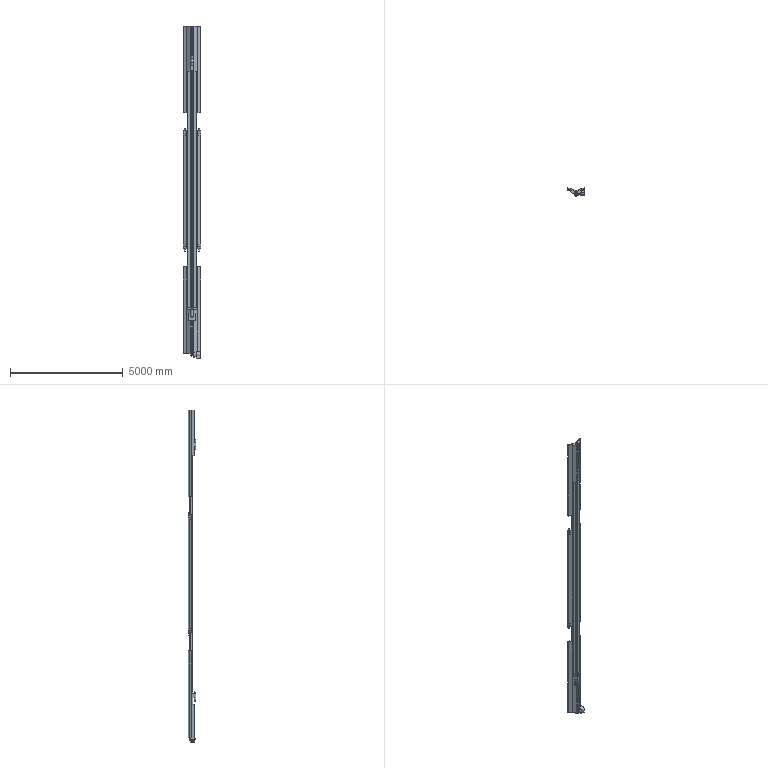Part | SolidWorks | features ICE 41, Extrusion 1 | 1 solid | 354 faces | box 771.866 x 352.673 x 14699 mm | volume 861943756 mm3 | plane 303 | cylinder 51 | commonest cylinder face diameters 70 x18 95 x14 35 x8 150 x3 80 x2 110 x2